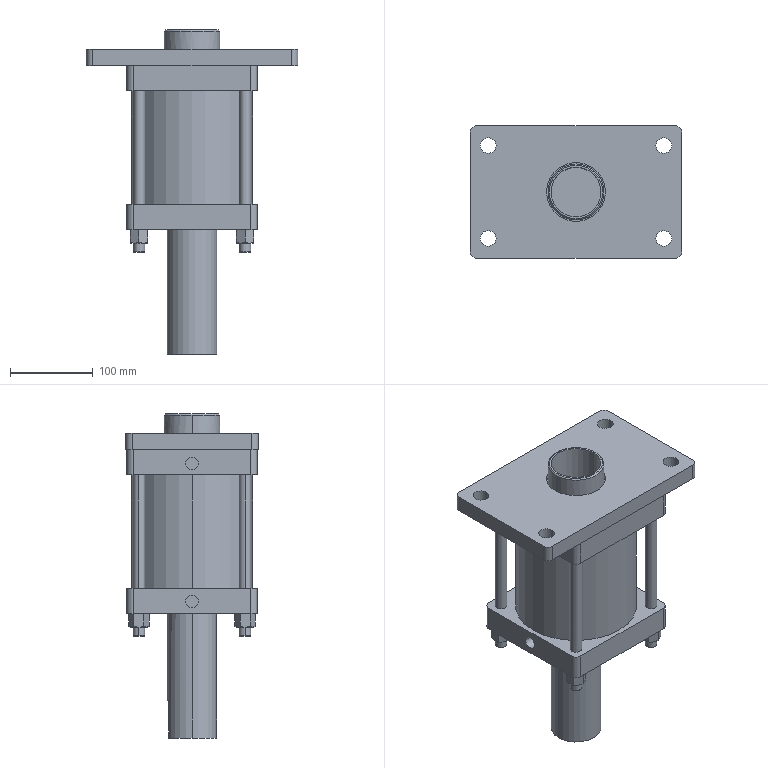Part | STEP file | 3 solids | 160 faces | box 255 x 160 x 391 mm | volume 4492396 mm3 | plane 64 | cylinder 60 | cone 36 | commonest cylinder face diameters 14 x16 15.7 x8 19 x8 7.381 x4 12.302 x4 15 x4